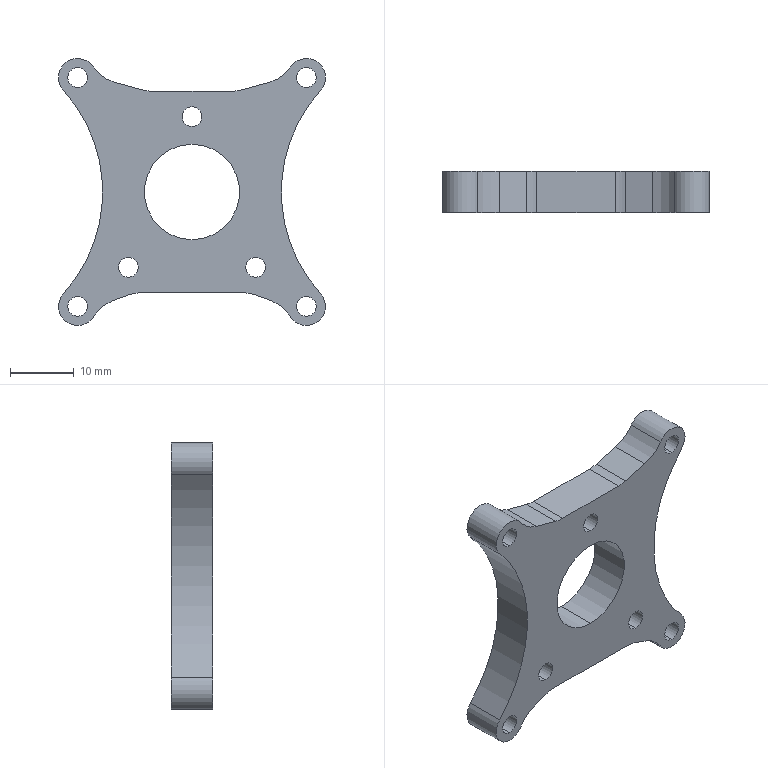Part | SolidWorks | features ICE 2, Extrusion 1, Fillet 1 | 1 solid | 49 faces | box 42 x 6.5 x 42 mm | volume 5775 mm3 | cylinder 38 | plane 11 | commonest cylinder face diameters 3.1 x14 6 x12 12 x8 15 x2 47.629 x2